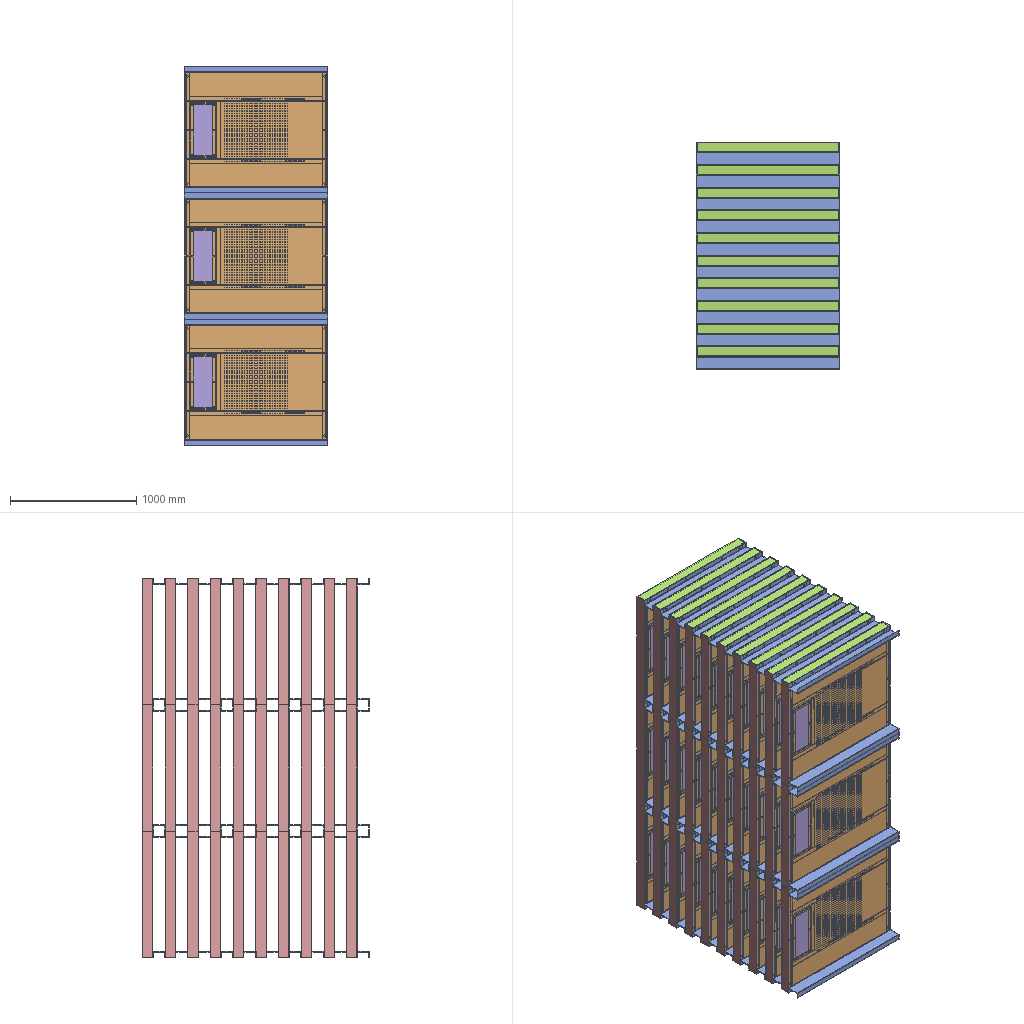Assembly | SolidWorks | 9 different items | 361 placed | box 1140 x 1800 x 3000 mm
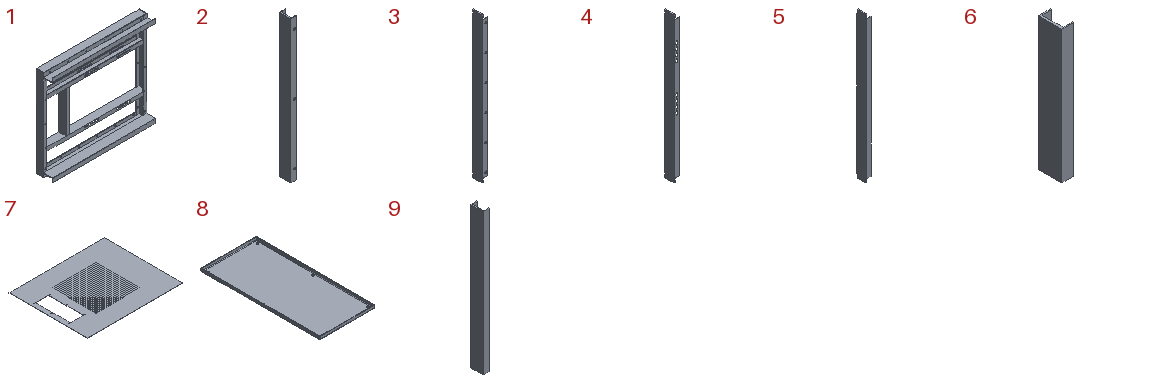Parts list (item | name | quantity | parent item | size | volume | features):
1 | (subassembly) | x30 | - | 1140 x 180 x 1000 mm | 8629233 mm3 | -
2 | - | x60 | in 1 | 40 x 80 x 1000 mm | 892305 mm3 | features Extrusion 1, ICE 1, LPattern 1, SheetMetal 1
3 | - | x60 | in 1 | 40 x 80 x 1124 mm | 979235 mm3 | features Cut 2, Extrusion 1, ICE 1, LPattern 1, SheetMetal 1
4 | - | x60 | in 1 | 40 x 80 x 1124 mm | 962436 mm3 | features Cut 3, LPattern 2, Extrusion 1, SheetMetal 1
5 | - | x1 | - | 40 x 80 x 1232 mm | 1071667 mm3 | features Cut 3, LPattern 2, Extrusion 1, SheetMetal 1
6 | - | x30 | in 1 | 40 x 80 x 455 mm | 407680 mm3 | features Extrusion 1, SheetMetal 1
7 | - | x30 | - | 1100 x 904 x 2 mm | 1841113 mm3 | features Cut 3, LPattern 2, FlatPattern 1, SMBaseFlange 1, SheetMetal 1
8 | - | x30 | - | 200 x 430 x 12 mm | 193280 mm3 | features EdgeFlange 2, CornerFeat 1, Cut 1, FlatPattern 1, LPattern 1, SMBaseFlange 1, SheetMetal 1
9 | - | x60 | in 1 | 48 x 100 x 1140 mm | 1276800 mm3 | features Extrusion 1, SheetMetal 1
Mates (type | each side: item.copy, entity, surface, feature):
In the top assembly
Coincident | 4.1 face plane Extrude1 | 7.1 face plane Base-Flange1
Coincident | 9.1 face plane Extrude1 | 7.1 face plane Base-Flange1
DistanceDim | 7.1 edge | 2.1 face plane Extrude1
Concentric | 7.1 face cylinder LPattern2 | 8.1 face cylinder LPattern1
Concentric | 7.1 face cylinder Cut-Extrude3 | 8.1 face cylinder Cut-Extrude1
Coincident | 7.1 face plane Base-Flange1 | 8.1 face plane Edge-Flange2
In subassembly 1
Coincident | 2.2 face plane Extrude1 | 3.1 face plane Extrude1 | 3 times
Coincident | 3.1 face plane Extrude1 | 2.3 face plane Extrude1 | 3 times
Coincident | 2.2 face plane Extrude1 | 3.2 face plane Extrude1 | 3 times
Coincident | 9.2 face plane Extrude1 | 3.2 face plane Extrude1 | 2 times
Coincident | 9.2 face plane Extrude1 | 2.3 face plane Extrude1
Coincident | 3.1 face plane Extrude1 | 9.3 face plane Extrude1 | 2 times
Coincident | 2.2 face plane Extrude1 | 9.3 face plane Extrude1
Coincident | 2.3 face plane Extrude1 | 4.2 face plane Extrude1 | 2 times
Coincident | 6.1 face plane Extrude1 | 4.2 face plane Extrude1 | 2 times
Coincident | 6.1 face plane Extrude1 | 4.3 face plane Extrude1 | 2 times
Coincident | 2.2 face plane Extrude1 | 4.3 face plane Extrude1
DistanceDim | 6.1 face plane Extrude1 | 2.2 face plane Extrude1
DistanceDim | 4.2 face plane Extrude1 | 3.2 face plane Extrude1